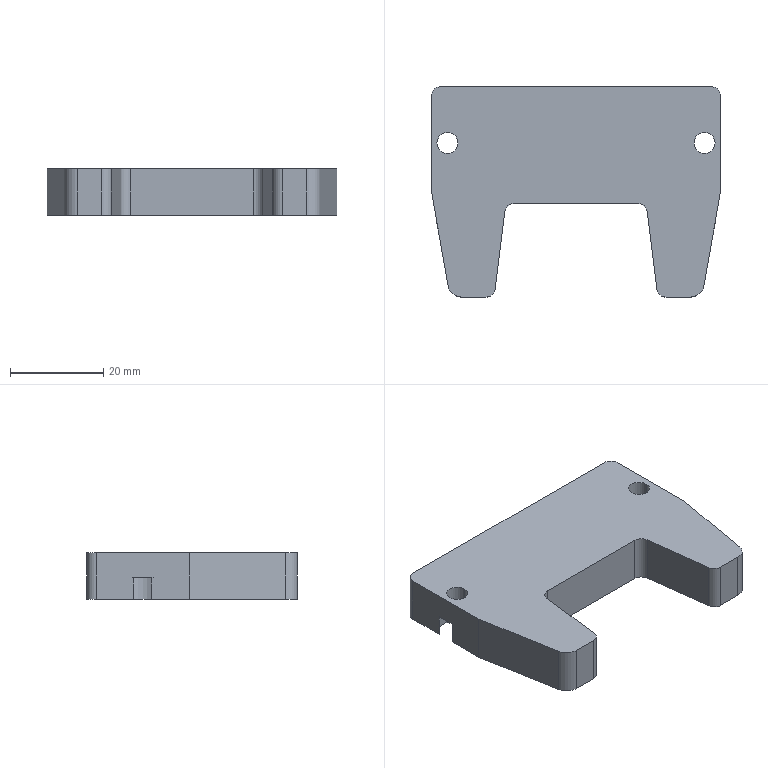Part | SolidWorks | features BaseBody 1 | 1 solid | 29 faces | box 62 x 45 x 10 mm | volume 19803 mm3 | cylinder 15 | plane 14 | commonest cylinder face diameters 4 x6 4.5 x4 8 x3 6 x2
STEP:
#1=CARTESIAN_POINT('',(-25.25,10.5,10.));
#2=VERTEX_POINT('',#1);
#3=CARTESIAN_POINT('',(-25.25,10.5,4.6));
#4=VERTEX_POINT('',#3);
#5=CARTESIAN_POINT('',(-25.25,10.5,0.));
#6=DIRECTION('',(0.,0.,-1.));
#7=VECTOR('',#6,1000.);
#8=LINE('',#5,#7);
#9=EDGE_CURVE('',#2,#4,#8,.T.);
#10=ORIENTED_EDGE('',*,*,#9,.F.);
#11=CARTESIAN_POINT('',(-29.75,10.5,10.));
#12=VERTEX_POINT('',#11);
#13=CARTESIAN_POINT('',(-27.5,10.5,10.));
#14=DIRECTION('',(0.,0.,1.));
#15=DIRECTION('',(1.,0.,0.));
#16=AXIS2_PLACEMENT_3D('',#13,#14,#15);
#17=CIRCLE('',#16,2.25);
#18=EDGE_CURVE('',#2,#12,#17,.T.);
#19=ORIENTED_EDGE('',*,*,#18,.T.);
#20=CARTESIAN_POINT('',(-29.75,10.5,4.6));
#21=VERTEX_POINT('',#20);
#22=CARTESIAN_POINT('',(-29.75,10.5,0.));
#23=DIRECTION('',(0.,0.,-1.));
#24=VECTOR('',#23,1000.);
#25=LINE('',#22,#24);
#26=EDGE_CURVE('',#12,#21,#25,.T.);
#27=ORIENTED_EDGE('',*,*,#26,.T.);
#28=CARTESIAN_POINT('',(-27.5,10.5,4.6));
#29=DIRECTION('',(0.,0.,-1.));
#30=DIRECTION('',(-1.,0.,0.));
#31=AXIS2_PLACEMENT_3D('',#28,#29,#30);
#32=CIRCLE('',#31,2.25);
#33=EDGE_CURVE('',#21,#4,#32,.T.);
#34=ORIENTED_EDGE('',*,*,#33,.T.);
#35=EDGE_LOOP('',(#10,#19,#27,#34));
#36=FACE_OUTER_BOUND('',#35,.T.);
#37=CARTESIAN_POINT('',(-27.5,10.5,0.));
#38=DIRECTION('',(0.,0.,-1.));
#39=DIRECTION('',(-1.,0.,0.));
#40=AXIS2_PLACEMENT_3D('',#37,#38,#39);
#41=CYLINDRICAL_SURFACE('',#40,2.25);
#42=ADVANCED_FACE('',(#36),#41,.F.);
#43=CARTESIAN_POINT('',(-31.,12.436,4.6));
#44=VERTEX_POINT('',#43);
#45=CARTESIAN_POINT('',(-31.,8.564,4.6));
#46=VERTEX_POINT('',#45);
#47=CARTESIAN_POINT('',(-27.5,10.5,4.6));
#48=DIRECTION('',(0.,0.,-1.));
#49=DIRECTION('',(-1.,0.,0.));
#50=AXIS2_PLACEMENT_3D('',#47,#48,#49);
#51=CIRCLE('',#50,4.);
#52=EDGE_CURVE('',#44,#46,#51,.T.);
#53=ORIENTED_EDGE('',*,*,#52,.F.);
#54=CARTESIAN_POINT('',(-31.,12.436,0.));
#55=VERTEX_POINT('',#54);
#56=CARTESIAN_POINT('',(-31.,12.436,0.));
#57=DIRECTION('',(0.,0.,1.));
#58=VECTOR('',#57,1000.);
#59=LINE('',#56,#58);
#60=EDGE_CURVE('',#55,#44,#59,.T.);
#61=ORIENTED_EDGE('',*,*,#60,.F.);
#62=CARTESIAN_POINT('',(-31.,8.564,0.));
#63=VERTEX_POINT('',#62);
#64=CARTESIAN_POINT('',(-27.5,10.5,0.));
#65=DIRECTION('',(0.,0.,-1.));
#66=DIRECTION('',(-1.,0.,0.));
#67=AXIS2_PLACEMENT_3D('',#64,#65,#66);
#68=CIRCLE('',#67,4.);
#69=EDGE_CURVE('',#55,#63,#68,.T.);
#70=ORIENTED_EDGE('',*,*,#69,.T.);
#71=CARTESIAN_POINT('',(-31.,8.564,0.));
#72=DIRECTION('',(0.,0.,-1.));
#73=VECTOR('',#72,1000.);
#74=LINE('',#71,#73);
#75=EDGE_CURVE('',#46,#63,#74,.T.);
#76=ORIENTED_EDGE('',*,*,#75,.F.);
#77=EDGE_LOOP('',(#53,#61,#70,#76));
#78=FACE_OUTER_BOUND('',#77,.T.);
#79=CARTESIAN_POINT('',(-27.5,10.5,0.));
#80=DIRECTION('',(0.,0.,-1.));
#81=DIRECTION('',(-1.,0.,0.));
#82=AXIS2_PLACEMENT_3D('',#79,#80,#81);
#83=CYLINDRICAL_SURFACE('',#82,4.);
#84=ADVANCED_FACE('',(#78),#83,.F.);
#85=ORIENTED_EDGE('',*,*,#33,.F.);
#86=CARTESIAN_POINT('',(-27.5,10.5,4.6));
#87=DIRECTION('',(0.,0.,-1.));
#88=DIRECTION('',(-1.,0.,0.));
#89=AXIS2_PLACEMENT_3D('',#86,#87,#88);
#90=CIRCLE('',#89,2.25);
#91=EDGE_CURVE('',#4,#21,#90,.T.);
#92=ORIENTED_EDGE('',*,*,#91,.F.);
#93=EDGE_LOOP('',(#85,#92));
#94=FACE_BOUND('',#93,.T.);
#95=ORIENTED_EDGE('',*,*,#52,.T.);
#96=CARTESIAN_POINT('',(-31.,-22.5,4.6));
#97=DIRECTION('',(0.,-1.,0.));
#98=VECTOR('',#97,1000.);
#99=LINE('',#96,#98);
#100=EDGE_CURVE('',#44,#46,#99,.T.);
#101=ORIENTED_EDGE('',*,*,#100,.F.);
#102=EDGE_LOOP('',(#95,#101));
#103=FACE_OUTER_BOUND('',#102,.T.);
#104=CARTESIAN_POINT('',(-25.25,10.5,4.6));
#105=DIRECTION('',(0.,0.,1.));
#106=DIRECTION('',(1.,0.,0.));
#107=AXIS2_PLACEMENT_3D('',#104,#105,#106);
#108=PLANE('',#107);
#109=ADVANCED_FACE('',(#94,#103),#108,.F.);
#110=CARTESIAN_POINT('',(29.75,10.5,10.));
#111=VERTEX_POINT('',#110);
#112=CARTESIAN_POINT('',(29.75,10.5,4.6));
#113=VERTEX_POINT('',#112);
#114=CARTESIAN_POINT('',(29.75,10.5,0.));
#115=DIRECTION('',(0.,0.,-1.));
#116=VECTOR('',#115,1000.);
#117=LINE('',#114,#116);
#118=EDGE_CURVE('',#111,#113,#117,.T.);
#119=ORIENTED_EDGE('',*,*,#118,.F.);
#120=CARTESIAN_POINT('',(25.25,10.5,10.));
#121=VERTEX_POINT('',#120);
#122=CARTESIAN_POINT('',(27.5,10.5,10.));
#123=DIRECTION('',(0.,0.,1.));
#124=DIRECTION('',(1.,0.,0.));
#125=AXIS2_PLACEMENT_3D('',#122,#123,#124);
#126=CIRCLE('',#125,2.25);
#127=EDGE_CURVE('',#111,#121,#126,.T.);
#128=ORIENTED_EDGE('',*,*,#127,.T.);
#129=CARTESIAN_POINT('',(25.25,10.5,4.6));
#130=VERTEX_POINT('',#129);
#131=CARTESIAN_POINT('',(25.25,10.5,0.));
#132=DIRECTION('',(0.,0.,-1.));
#133=VECTOR('',#132,1000.);
#134=LINE('',#131,#133);
#135=EDGE_CURVE('',#121,#130,#134,.T.);
#136=ORIENTED_EDGE('',*,*,#135,.T.);
#137=CARTESIAN_POINT('',(27.5,10.5,4.6));
#138=DIRECTION('',(0.,0.,-1.));
#139=DIRECTION('',(-1.,0.,0.));
#140=AXIS2_PLACEMENT_3D('',#137,#138,#139);
#141=CIRCLE('',#140,2.25);
#142=EDGE_CURVE('',#130,#113,#141,.T.);
#143=ORIENTED_EDGE('',*,*,#142,.T.);
#144=EDGE_LOOP('',(#119,#128,#136,#143));
#145=FACE_OUTER_BOUND('',#144,.T.);
#146=CARTESIAN_POINT('',(27.5,10.5,0.));
#147=DIRECTION('',(0.,0.,-1.));
#148=DIRECTION('',(-1.,0.,0.));
#149=AXIS2_PLACEMENT_3D('',#146,#147,#148);
#150=CYLINDRICAL_SURFACE('',#149,2.25);
#151=ADVANCED_FACE('',(#145),#150,.F.);
#152=CARTESIAN_POINT('',(23.5,10.5,4.6));
#153=VERTEX_POINT('',#152);
#154=CARTESIAN_POINT('',(23.5,10.5,0.));
#155=VERTEX_POINT('',#154);
#156=CARTESIAN_POINT('',(23.5,10.5,0.));
#157=DIRECTION('',(0.,0.,-1.));
#158=VECTOR('',#157,1000.);
#159=LINE('',#156,#158);
#160=EDGE_CURVE('',#153,#155,#159,.T.);
#161=ORIENTED_EDGE('',*,*,#160,.F.);
#162=CARTESIAN_POINT('',(31.,8.564,4.6));
#163=VERTEX_POINT('',#162);
#164=CARTESIAN_POINT('',(27.5,10.5,4.6));
#165=DIRECTION('',(0.,0.,-1.));
#166=DIRECTION('',(-1.,0.,0.));
#167=AXIS2_PLACEMENT_3D('',#164,#165,#166);
#168=CIRCLE('',#167,4.);
#169=EDGE_CURVE('',#163,#153,#168,.T.);
#170=ORIENTED_EDGE('',*,*,#169,.F.);
#171=CARTESIAN_POINT('',(31.,8.564,0.));
#172=VERTEX_POINT('',#171);
#173=CARTESIAN_POINT('',(31.,8.564,0.));
#174=DIRECTION('',(0.,0.,1.));
#175=VECTOR('',#174,1000.);
#176=LINE('',#173,#175);
#177=EDGE_CURVE('',#172,#163,#176,.T.);
#178=ORIENTED_EDGE('',*,*,#177,.F.);
#179=CARTESIAN_POINT('',(27.5,10.5,0.));
#180=DIRECTION('',(0.,0.,-1.));
#181=DIRECTION('',(-1.,0.,0.));
#182=AXIS2_PLACEMENT_3D('',#179,#180,#181);
#183=CIRCLE('',#182,4.);
#184=EDGE_CURVE('',#172,#155,#183,.T.);
#185=ORIENTED_EDGE('',*,*,#184,.T.);
#186=EDGE_LOOP('',(#161,#170,#178,#185));
#187=FACE_OUTER_BOUND('',#186,.T.);
#188=CARTESIAN_POINT('',(27.5,10.5,0.));
#189=DIRECTION('',(0.,0.,-1.));
#190=DIRECTION('',(-1.,0.,0.));
#191=AXIS2_PLACEMENT_3D('',#188,#189,#190);
#192=CYLINDRICAL_SURFACE('',#191,4.);
#193=ADVANCED_FACE('',(#187),#192,.F.);
#194=ORIENTED_EDGE('',*,*,#142,.F.);
#195=CARTESIAN_POINT('',(27.5,10.5,4.6));
#196=DIRECTION('',(0.,0.,-1.));
#197=DIRECTION('',(-1.,0.,0.));
#198=AXIS2_PLACEMENT_3D('',#195,#196,#197);
#199=CIRCLE('',#198,2.25);
#200=EDGE_CURVE('',#113,#130,#199,.T.);
#201=ORIENTED_EDGE('',*,*,#200,.F.);
#202=EDGE_LOOP('',(#194,#201));
#203=FACE_BOUND('',#202,.T.);
#204=ORIENTED_EDGE('',*,*,#169,.T.);
#205=CARTESIAN_POINT('',(31.,12.436,4.6));
#206=VERTEX_POINT('',#205);
#207=CARTESIAN_POINT('',(27.5,10.5,4.6));
#208=DIRECTION('',(0.,0.,-1.));
#209=DIRECTION('',(-1.,0.,0.));
#210=AXIS2_PLACEMENT_3D('',#207,#208,#209);
#211=CIRCLE('',#210,4.);
#212=EDGE_CURVE('',#153,#206,#211,.T.);
#213=ORIENTED_EDGE('',*,*,#212,.T.);
#214=CARTESIAN_POINT('',(31.,-22.5,4.6));
#215=DIRECTION('',(0.,1.,0.));
#216=VECTOR('',#215,1000.);
#217=LINE('',#214,#216);
#218=EDGE_CURVE('',#163,#206,#217,.T.);
#219=ORIENTED_EDGE('',*,*,#218,.F.);
#220=EDGE_LOOP('',(#204,#213,#219));
#221=FACE_OUTER_BOUND('',#220,.T.);
#222=CARTESIAN_POINT('',(29.75,10.5,4.6));
#223=DIRECTION('',(0.,0.,1.));
#224=DIRECTION('',(1.,0.,0.));
#225=AXIS2_PLACEMENT_3D('',#222,#223,#224);
#226=PLANE('',#225);
#227=ADVANCED_FACE('',(#203,#221),#226,.F.);
#228=CARTESIAN_POINT('',(-27.382,-20.021,10.));
#229=VERTEX_POINT('',#228);
#230=CARTESIAN_POINT('',(-24.427,-22.5,10.));
#231=VERTEX_POINT('',#230);
#232=CARTESIAN_POINT('',(-24.427,-19.5,10.));
#233=DIRECTION('',(0.,0.,1.));
#234=DIRECTION('',(1.,0.,0.));
#235=AXIS2_PLACEMENT_3D('',#232,#233,#234);
#236=CIRCLE('',#235,3.);
#237=EDGE_CURVE('',#229,#231,#236,.T.);
#238=ORIENTED_EDGE('',*,*,#237,.F.);
#239=CARTESIAN_POINT('',(-27.382,-20.021,0.));
#240=VERTEX_POINT('',#239);
#241=CARTESIAN_POINT('',(-27.382,-20.021,10.));
#242=DIRECTION('',(0.,0.,1.));
#243=VECTOR('',#242,1000.);
#244=LINE('',#241,#243);
#245=EDGE_CURVE('',#240,#229,#244,.T.);
#246=ORIENTED_EDGE('',*,*,#245,.F.);
#247=CARTESIAN_POINT('',(-24.427,-22.5,0.));
#248=VERTEX_POINT('',#247);
#249=CARTESIAN_POINT('',(-24.427,-19.5,0.));
#250=DIRECTION('',(0.,0.,-1.));
#251=DIRECTION('',(1.,0.,0.));
#252=AXIS2_PLACEMENT_3D('',#249,#250,#251);
#253=CIRCLE('',#252,3.);
#254=EDGE_CURVE('',#248,#240,#253,.T.);
#255=ORIENTED_EDGE('',*,*,#254,.F.);
#256=CARTESIAN_POINT('',(-24.427,-22.5,0.));
#257=DIRECTION('',(0.,0.,-1.));
#258=VECTOR('',#257,1000.);
#259=LINE('',#256,#258);
#260=EDGE_CURVE('',#231,#248,#259,.T.);
#261=ORIENTED_EDGE('',*,*,#260,.F.);
#262=EDGE_LOOP('',(#238,#246,#255,#261));
#263=FACE_OUTER_BOUND('',#262,.T.);
#264=CARTESIAN_POINT('',(-24.427,-19.5,10.));
#265=DIRECTION('',(0.,0.,-1.));
#266=DIRECTION('',(-1.,0.,0.));
#267=AXIS2_PLACEMENT_3D('',#264,#265,#266);
#268=CYLINDRICAL_SURFACE('',#267,3.);
#269=ADVANCED_FACE('',(#263),#268,.T.);
#270=CARTESIAN_POINT('',(27.382,-20.021,0.));
#271=VERTEX_POINT('',#270);
#272=CARTESIAN_POINT('',(24.427,-22.5,0.));
#273=VERTEX_POINT('',#272);
#274=CARTESIAN_POINT('',(24.427,-19.5,0.));
#275=DIRECTION('',(0.,0.,-1.));
#276=DIRECTION('',(1.,0.,0.));
#277=AXIS2_PLACEMENT_3D('',#274,#275,#276);
#278=CIRCLE('',#277,3.);
#279=EDGE_CURVE('',#271,#273,#278,.T.);
#280=ORIENTED_EDGE('',*,*,#279,.F.);
#281=CARTESIAN_POINT('',(27.382,-20.021,10.));
#282=VERTEX_POINT('',#281);
#283=CARTESIAN_POINT('',(27.382,-20.021,0.));
#284=DIRECTION('',(0.,0.,-1.));
#285=VECTOR('',#284,1000.);
#286=LINE('',#283,#285);
#287=EDGE_CURVE('',#282,#271,#286,.T.);
#288=ORIENTED_EDGE('',*,*,#287,.F.);
#289=CARTESIAN_POINT('',(24.427,-22.5,10.));
#290=VERTEX_POINT('',#289);
#291=CARTESIAN_POINT('',(24.427,-19.5,10.));
#292=DIRECTION('',(0.,0.,1.));
#293=DIRECTION('',(1.,0.,0.));
#294=AXIS2_PLACEMENT_3D('',#291,#292,#293);
#295=CIRCLE('',#294,3.);
#296=EDGE_CURVE('',#290,#282,#295,.T.);
#297=ORIENTED_EDGE('',*,*,#296,.F.);
#298=CARTESIAN_POINT('',(24.427,-22.5,10.));
#299=DIRECTION('',(0.,0.,1.));
#300=VECTOR('',#299,1000.);
#301=LINE('',#298,#300);
#302=EDGE_CURVE('',#273,#290,#301,.T.);
#303=ORIENTED_EDGE('',*,*,#302,.F.);
#304=EDGE_LOOP('',(#280,#288,#297,#303));
#305=FACE_OUTER_BOUND('',#304,.T.);
#306=CARTESIAN_POINT('',(24.427,-19.5,10.));
#307=DIRECTION('',(0.,0.,1.));
#308=DIRECTION('',(1.,0.,0.));
#309=AXIS2_PLACEMENT_3D('',#306,#307,#308);
#310=CYLINDRICAL_SURFACE('',#309,3.);
#311=ADVANCED_FACE('',(#305),#310,.T.);
#312=CARTESIAN_POINT('',(-31.,0.5,0.));
#313=VERTEX_POINT('',#312);
#314=CARTESIAN_POINT('',(-26.944,-22.5,0.));
#315=DIRECTION('',(-0.1736,0.9848,0.));
#316=VECTOR('',#315,1000.);
#317=LINE('',#314,#316);
#318=EDGE_CURVE('',#240,#313,#317,.T.);
#319=ORIENTED_EDGE('',*,*,#318,.F.);
#320=ORIENTED_EDGE('',*,*,#245,.T.);
#321=CARTESIAN_POINT('',(-31.,0.5,10.));
#322=VERTEX_POINT('',#321);
#323=CARTESIAN_POINT('',(-29.98,-5.286,10.));
#324=DIRECTION('',(0.1736,-0.9848,0.));
#325=VECTOR('',#324,1000.);
#326=LINE('',#323,#325);
#327=EDGE_CURVE('',#322,#229,#326,.T.);
#328=ORIENTED_EDGE('',*,*,#327,.F.);
#329=CARTESIAN_POINT('',(-31.,0.5,10.));
#330=DIRECTION('',(0.,0.,1.));
#331=VECTOR('',#330,1000.);
#332=LINE('',#329,#331);
#333=EDGE_CURVE('',#313,#322,#332,.T.);
#334=ORIENTED_EDGE('',*,*,#333,.F.);
#335=EDGE_LOOP('',(#319,#320,#328,#334));
#336=FACE_OUTER_BOUND('',#335,.T.);
#337=CARTESIAN_POINT('',(-26.944,-22.5,10.));
#338=DIRECTION('',(0.9848,0.1736,0.));
#339=DIRECTION('',(0.,0.,-1.));
#340=AXIS2_PLACEMENT_3D('',#337,#338,#339);
#341=PLANE('',#340);
#342=ADVANCED_FACE('',(#336),#341,.F.);
#343=CARTESIAN_POINT('',(31.,0.5,10.));
#344=VERTEX_POINT('',#343);
#345=CARTESIAN_POINT('',(29.98,-5.286,10.));
#346=DIRECTION('',(0.1736,0.9848,0.));
#347=VECTOR('',#346,1000.);
#348=LINE('',#345,#347);
#349=EDGE_CURVE('',#282,#344,#348,.T.);
#350=ORIENTED_EDGE('',*,*,#349,.F.);
#351=ORIENTED_EDGE('',*,*,#287,.T.);
#352=CARTESIAN_POINT('',(31.,0.5,0.));
#353=VERTEX_POINT('',#352);
#354=CARTESIAN_POINT('',(31.,0.5,0.));
#355=DIRECTION('',(-0.1736,-0.9848,0.));
#356=VECTOR('',#355,1000.);
#357=LINE('',#354,#356);
#358=EDGE_CURVE('',#353,#271,#357,.T.);
#359=ORIENTED_EDGE('',*,*,#358,.F.);
#360=CARTESIAN_POINT('',(31.,0.5,10.));
#361=DIRECTION('',(0.,0.,-1.));
#362=VECTOR('',#361,1000.);
#363=LINE('',#360,#362);
#364=EDGE_CURVE('',#344,#353,#363,.T.);
#365=ORIENTED_EDGE('',*,*,#364,.F.);
#366=EDGE_LOOP('',(#350,#351,#359,#365));
#367=FACE_OUTER_BOUND('',#366,.T.);
#368=CARTESIAN_POINT('',(31.,0.5,10.));
#369=DIRECTION('',(-0.9848,0.1736,0.));
#370=DIRECTION('',(0.,0.,1.));
#371=AXIS2_PLACEMENT_3D('',#368,#369,#370);
#372=PLANE('',#371);
#373=ADVANCED_FACE('',(#367),#372,.F.);
#374=CARTESIAN_POINT('',(-13.234,-2.5,0.));
#375=VERTEX_POINT('',#374);
#376=CARTESIAN_POINT('',(-15.219,-4.252,0.));
#377=VERTEX_POINT('',#376);
#378=CARTESIAN_POINT('',(-13.234,-4.5,0.));
#379=DIRECTION('',(0.,0.,1.));
#380=DIRECTION('',(1.,0.,0.));
#381=AXIS2_PLACEMENT_3D('',#378,#379,#380);
#382=CIRCLE('',#381,2.);
#383=EDGE_CURVE('',#375,#377,#382,.T.);
#384=ORIENTED_EDGE('',*,*,#383,.F.);
#385=CARTESIAN_POINT('',(-13.234,-2.5,10.));
#386=VERTEX_POINT('',#385);
#387=CARTESIAN_POINT('',(-13.234,-2.5,0.));
#388=DIRECTION('',(0.,0.,-1.));
#389=VECTOR('',#388,1000.);
#390=LINE('',#387,#389);
#391=EDGE_CURVE('',#386,#375,#390,.T.);
#392=ORIENTED_EDGE('',*,*,#391,.F.);
#393=CARTESIAN_POINT('',(-15.219,-4.252,10.));
#394=VERTEX_POINT('',#393);
#395=CARTESIAN_POINT('',(-13.234,-4.5,10.));
#396=DIRECTION('',(0.,0.,-1.));
#397=DIRECTION('',(1.,0.,0.));
#398=AXIS2_PLACEMENT_3D('',#395,#396,#397);
#399=CIRCLE('',#398,2.);
#400=EDGE_CURVE('',#394,#386,#399,.T.);
#401=ORIENTED_EDGE('',*,*,#400,.F.);
#402=CARTESIAN_POINT('',(-15.219,-4.252,10.));
#403=DIRECTION('',(0.,0.,1.));
#404=VECTOR('',#403,1000.);
#405=LINE('',#402,#404);
#406=EDGE_CURVE('',#377,#394,#405,.T.);
#407=ORIENTED_EDGE('',*,*,#406,.F.);
#408=EDGE_LOOP('',(#384,#392,#401,#407));
#409=FACE_OUTER_BOUND('',#408,.T.);
#410=CARTESIAN_POINT('',(-13.234,-4.5,-0.001));
#411=DIRECTION('',(0.,0.,-1.));
#412=DIRECTION('',(-1.,0.,0.));
#413=AXIS2_PLACEMENT_3D('',#410,#411,#412);
#414=CYLINDRICAL_SURFACE('',#413,2.);
#415=ADVANCED_FACE('',(#409),#414,.F.);
#416=CARTESIAN_POINT('',(15.219,-4.252,0.));
#417=VERTEX_POINT('',#416);
#418=CARTESIAN_POINT('',(13.234,-2.5,0.));
#419=VERTEX_POINT('',#418);
#420=CARTESIAN_POINT('',(13.234,-4.5,0.));
#421=DIRECTION('',(0.,0.,1.));
#422=DIRECTION('',(1.,0.,0.));
#423=AXIS2_PLACEMENT_3D('',#420,#421,#422);
#424=CIRCLE('',#423,2.);
#425=EDGE_CURVE('',#417,#419,#424,.T.);
#426=ORIENTED_EDGE('',*,*,#425,.F.);
#427=CARTESIAN_POINT('',(15.219,-4.252,10.));
#428=VERTEX_POINT('',#427);
#429=CARTESIAN_POINT('',(15.219,-4.252,0.));
#430=DIRECTION('',(0.,0.,-1.));
#431=VECTOR('',#430,1000.);
#432=LINE('',#429,#431);
#433=EDGE_CURVE('',#428,#417,#432,.T.);
#434=ORIENTED_EDGE('',*,*,#433,.F.);
#435=CARTESIAN_POINT('',(13.234,-2.5,10.));
#436=VERTEX_POINT('',#435);
#437=CARTESIAN_POINT('',(13.234,-4.5,10.));
#438=DIRECTION('',(0.,0.,-1.));
#439=DIRECTION('',(1.,0.,0.));
#440=AXIS2_PLACEMENT_3D('',#437,#438,#439);
#441=CIRCLE('',#440,2.);
#442=EDGE_CURVE('',#436,#428,#441,.T.);
#443=ORIENTED_EDGE('',*,*,#442,.F.);
#444=CARTESIAN_POINT('',(13.234,-2.5,10.));
#445=DIRECTION('',(0.,0.,1.));
#446=VECTOR('',#445,1000.);
#447=LINE('',#444,#446);
#448=EDGE_CURVE('',#419,#436,#447,.T.);
#449=ORIENTED_EDGE('',*,*,#448,.F.);
#450=EDGE_LOOP('',(#426,#434,#443,#449));
#451=FACE_OUTER_BOUND('',#450,.T.);
#452=CARTESIAN_POINT('',(13.234,-4.5,-0.001));
#453=DIRECTION('',(0.,0.,-1.));
#454=DIRECTION('',(-1.,0.,0.));
#455=AXIS2_PLACEMENT_3D('',#452,#453,#454);
#456=CYLINDRICAL_SURFACE('',#455,2.);
#457=ADVANCED_FACE('',(#451),#456,.F.);
#458=CARTESIAN_POINT('',(-17.281,-20.748,0.));
#459=VERTEX_POINT('',#458);
#460=CARTESIAN_POINT('',(-19.266,-22.5,0.));
#461=VERTEX_POINT('',#460);
#462=CARTESIAN_POINT('',(-19.266,-20.5,0.));
#463=DIRECTION('',(0.,0.,-1.));
#464=DIRECTION('',(1.,0.,0.));
#465=AXIS2_PLACEMENT_3D('',#462,#463,#464);
#466=CIRCLE('',#465,2.);
#467=EDGE_CURVE('',#459,#461,#466,.T.);
#468=ORIENTED_EDGE('',*,*,#467,.F.);
#469=CARTESIAN_POINT('',(-17.281,-20.748,10.));
#470=VERTEX_POINT('',#469);
#471=CARTESIAN_POINT('',(-17.281,-20.748,-0.001));
#472=DIRECTION('',(0.,0.,-1.));
#473=VECTOR('',#472,1000.);
#474=LINE('',#471,#473);
#475=EDGE_CURVE('',#470,#459,#474,.T.);
#476=ORIENTED_EDGE('',*,*,#475,.F.);
#477=CARTESIAN_POINT('',(-19.266,-22.5,10.));
#478=VERTEX_POINT('',#477);
#479=CARTESIAN_POINT('',(-19.266,-20.5,10.));
#480=DIRECTION('',(0.,0.,1.));
#481=DIRECTION('',(1.,0.,0.));
#482=AXIS2_PLACEMENT_3D('',#479,#480,#481);
#483=CIRCLE('',#482,2.);
#484=EDGE_CURVE('',#478,#470,#483,.T.);
#485=ORIENTED_EDGE('',*,*,#484,.F.);
#486=CARTESIAN_POINT('',(-19.266,-22.5,10.));
#487=DIRECTION('',(0.,0.,1.));
#488=VECTOR('',#487,1000.);
#489=LINE('',#486,#488);
#490=EDGE_CURVE('',#461,#478,#489,.T.);
#491=ORIENTED_EDGE('',*,*,#490,.F.);
#492=EDGE_LOOP('',(#468,#476,#485,#491));
#493=FACE_OUTER_BOUND('',#492,.T.);
#494=CARTESIAN_POINT('',(-19.266,-20.5,10.));
#495=DIRECTION('',(0.,0.,1.));
#496=DIRECTION('',(1.,0.,0.));
#497=AXIS2_PLACEMENT_3D('',#494,#495,#496);
#498=CYLINDRICAL_SURFACE('',#497,2.);
#499=ADVANCED_FACE('',(#493),#498,.T.);
#500=CARTESIAN_POINT('',(19.266,-22.5,0.));
#501=VERTEX_POINT('',#500);
#502=CARTESIAN_POINT('',(17.281,-20.748,0.));
#503=VERTEX_POINT('',#502);
#504=CARTESIAN_POINT('',(19.266,-20.5,0.));
#505=DIRECTION('',(0.,0.,-1.));
#506=DIRECTION('',(1.,0.,0.));
#507=AXIS2_PLACEMENT_3D('',#504,#505,#506);
#508=CIRCLE('',#507,2.);
#509=EDGE_CURVE('',#501,#503,#508,.T.);
#510=ORIENTED_EDGE('',*,*,#509,.F.);
#511=CARTESIAN_POINT('',(19.266,-22.5,10.));
#512=VERTEX_POINT('',#511);
#513=CARTESIAN_POINT('',(19.266,-22.5,10.));
#514=DIRECTION('',(0.,0.,-1.));
#515=VECTOR('',#514,1000.);
#516=LINE('',#513,#515);
#517=EDGE_CURVE('',#512,#501,#516,.T.);
#518=ORIENTED_EDGE('',*,*,#517,.F.);
#519=CARTESIAN_POINT('',(17.281,-20.748,10.));
#520=VERTEX_POINT('',#519);
#521=CARTESIAN_POINT('',(19.266,-20.5,10.));
#522=DIRECTION('',(0.,0.,1.));
#523=DIRECTION('',(1.,0.,0.));
#524=AXIS2_PLACEMENT_3D('',#521,#522,#523);
#525=CIRCLE('',#524,2.);
#526=EDGE_CURVE('',#520,#512,#525,.T.);
#527=ORIENTED_EDGE('',*,*,#526,.F.);
#528=CARTESIAN_POINT('',(17.281,-20.748,-0.001));
#529=DIRECTION('',(0.,0.,1.));
#530=VECTOR('',#529,1000.);
#531=LINE('',#528,#530);
#532=EDGE_CURVE('',#503,#520,#531,.T.);
#533=ORIENTED_EDGE('',*,*,#532,.F.);
#534=EDGE_LOOP('',(#510,#518,#527,#533));
#535=FACE_OUTER_BOUND('',#534,.T.);
#536=CARTESIAN_POINT('',(19.266,-20.5,-0.001));
#537=DIRECTION('',(0.,0.,1.));
#538=DIRECTION('',(1.,0.,0.));
#539=AXIS2_PLACEMENT_3D('',#536,#537,#538);
#540=CYLINDRICAL_SURFACE('',#539,2.);
#541=ADVANCED_FACE('',(#535),#540,.T.);
#542=CARTESIAN_POINT('',(31.,20.5,10.));
#543=VERTEX_POINT('',#542);
#544=CARTESIAN_POINT('',(29.,22.5,10.));
#545=VERTEX_POINT('',#544);
#546=CARTESIAN_POINT('',(29.,20.5,10.));
#547=DIRECTION('',(0.,0.,1.));
#548=DIRECTION('',(1.,0.,0.));
#549=AXIS2_PLACEMENT_3D('',#546,#547,#548);
#550=CIRCLE('',#549,2.);
#551=EDGE_CURVE('',#543,#545,#550,.T.);
#552=ORIENTED_EDGE('',*,*,#551,.F.);
#553=CARTESIAN_POINT('',(31.,20.5,0.));
#554=VERTEX_POINT('',#553);
#555=CARTESIAN_POINT('',(31.,20.5,10.));
#556=DIRECTION('',(0.,0.,1.));
#557=VECTOR('',#556,1000.);
#558=LINE('',#555,#557);
#559=EDGE_CURVE('',#554,#543,#558,.T.);
#560=ORIENTED_EDGE('',*,*,#559,.F.);
#561=CARTESIAN_POINT('',(29.,22.5,0.));
#562=VERTEX_POINT('',#561);
#563=CARTESIAN_POINT('',(29.,20.5,0.));
#564=DIRECTION('',(0.,0.,-1.));
#565=DIRECTION('',(1.,0.,0.));
#566=AXIS2_PLACEMENT_3D('',#563,#564,#565);
#567=CIRCLE('',#566,2.);
#568=EDGE_CURVE('',#562,#554,#567,.T.);
#569=ORIENTED_EDGE('',*,*,#568,.F.);
#570=CARTESIAN_POINT('',(29.,22.5,10.));
#571=DIRECTION('',(0.,0.,-1.));
#572=VECTOR('',#571,1000.);
#573=LINE('',#570,#572);
#574=EDGE_CURVE('',#545,#562,#573,.T.);
#575=ORIENTED_EDGE('',*,*,#574,.F.);
#576=EDGE_LOOP('',(#552,#560,#569,#575));
#577=FACE_OUTER_BOUND('',#576,.T.);
#578=CARTESIAN_POINT('',(29.,20.5,10.));
#579=DIRECTION('',(0.,0.,-1.));
#580=DIRECTION('',(-1.,0.,0.));
#581=AXIS2_PLACEMENT_3D('',#578,#579,#580);
#582=CYLINDRICAL_SURFACE('',#581,2.);
#583=ADVANCED_FACE('',(#577),#582,.T.);
#584=CARTESIAN_POINT('',(-29.,22.5,10.));
#585=VERTEX_POINT('',#584);
#586=CARTESIAN_POINT('',(-31.,20.5,10.));
#587=VERTEX_POINT('',#586);
#588=CARTESIAN_POINT('',(-29.,20.5,10.));
#589=DIRECTION('',(0.,0.,1.));
#590=DIRECTION('',(1.,0.,0.));
#591=AXIS2_PLACEMENT_3D('',#588,#589,#590);
#592=CIRCLE('',#591,2.);
#593=EDGE_CURVE('',#585,#587,#592,.T.);
#594=ORIENTED_EDGE('',*,*,#593,.F.);
#595=CARTESIAN_POINT('',(-29.,22.5,0.));
#596=VERTEX_POINT('',#595);
#597=CARTESIAN_POINT('',(-29.,22.5,10.));
#598=DIRECTION('',(0.,0.,1.));
#599=VECTOR('',#598,1000.);
#600=LINE('',#597,#599);
#601=EDGE_CURVE('',#596,#585,#600,.T.);
#602=ORIENTED_EDGE('',*,*,#601,.F.);
#603=CARTESIAN_POINT('',(-31.,20.5,0.));
#604=VERTEX_POINT('',#603);
#605=CARTESIAN_POINT('',(-29.,20.5,0.));
#606=DIRECTION('',(0.,0.,-1.));
#607=DIRECTION('',(1.,0.,0.));
#608=AXIS2_PLACEMENT_3D('',#605,#606,#607);
#609=CIRCLE('',#608,2.);
#610=EDGE_CURVE('',#604,#596,#609,.T.);
#611=ORIENTED_EDGE('',*,*,#610,.F.);
#612=CARTESIAN_POINT('',(-31.,20.5,10.));
#613=DIRECTION('',(0.,0.,-1.));
#614=VECTOR('',#613,1000.);
#615=LINE('',#612,#614);
#616=EDGE_CURVE('',#587,#604,#615,.T.);
#617=ORIENTED_EDGE('',*,*,#616,.F.);
#618=EDGE_LOOP('',(#594,#602,#611,#617));
#619=FACE_OUTER_BOUND('',#618,.T.);
#620=CARTESIAN_POINT('',(-29.,20.5,10.));
#621=DIRECTION('',(0.,0.,-1.));
#622=DIRECTION('',(-1.,0.,0.));
#623=AXIS2_PLACEMENT_3D('',#620,#621,#622);
#624=CYLINDRICAL_SURFACE('',#623,2.);
#625=ADVANCED_FACE('',(#619),#624,.T.);
#626=CARTESIAN_POINT('',(17.5,-22.5,0.));
#627=DIRECTION('',(0.124,-0.9923,0.));
#628=VECTOR('',#627,1000.);
#629=LINE('',#626,#628);
#630=EDGE_CURVE('',#417,#503,#629,.T.);
#631=ORIENTED_EDGE('',*,*,#630,.T.);
#632=ORIENTED_EDGE('',*,*,#532,.T.);
#633=CARTESIAN_POINT('',(17.5,-22.5,10.));
#634=DIRECTION('',(-0.124,0.9923,0.));
#635=VECTOR('',#634,1000.);
#636=LINE('',#633,#635);
#637=EDGE_CURVE('',#520,#428,#636,.T.);
#638=ORIENTED_EDGE('',*,*,#637,.T.);
#639=ORIENTED_EDGE('',*,*,#433,.T.);
#640=EDGE_LOOP('',(#631,#632,#638,#639));
#641=FACE_OUTER_BOUND('',#640,.T.);
#642=CARTESIAN_POINT('',(17.5,-22.5,-0.001));
#643=DIRECTION('',(0.9923,0.124,0.));
#644=DIRECTION('',(0.,0.,-1.));
#645=AXIS2_PLACEMENT_3D('',#642,#643,#644);
#646=PLANE('',#645);
#647=ADVANCED_FACE('',(#641),#646,.F.);
#648=CARTESIAN_POINT('',(15.,-2.5,0.));
#649=DIRECTION('',(1.,0.,0.));
#650=VECTOR('',#649,1000.);
#651=LINE('',#648,#650);
#652=EDGE_CURVE('',#375,#419,#651,.T.);
#653=ORIENTED_EDGE('',*,*,#652,.T.);
#654=ORIENTED_EDGE('',*,*,#448,.T.);
#655=CARTESIAN_POINT('',(15.,-2.5,10.));
#656=DIRECTION('',(-1.,0.,0.));
#657=VECTOR('',#656,1000.);
#658=LINE('',#655,#657);
#659=EDGE_CURVE('',#436,#386,#658,.T.);
#660=ORIENTED_EDGE('',*,*,#659,.T.);
#661=ORIENTED_EDGE('',*,*,#391,.T.);
#662=EDGE_LOOP('',(#653,#654,#660,#661));
#663=FACE_OUTER_BOUND('',#662,.T.);
#664=CARTESIAN_POINT('',(15.,-2.5,-0.001));
#665=DIRECTION('',(0.,1.,0.));
#666=DIRECTION('',(1.,0.,0.));
#667=AXIS2_PLACEMENT_3D('',#664,#665,#666);
#668=PLANE('',#667);
#669=ADVANCED_FACE('',(#663),#668,.F.);
#670=CARTESIAN_POINT('',(-15.,-2.5,10.));
#671=DIRECTION('',(-0.124,-0.9923,0.));
#672=VECTOR('',#671,1000.);
#673=LINE('',#670,#672);
#674=EDGE_CURVE('',#394,#470,#673,.T.);
#675=ORIENTED_EDGE('',*,*,#674,.T.);
#676=ORIENTED_EDGE('',*,*,#475,.T.);
#677=CARTESIAN_POINT('',(-15.,-2.5,0.));
#678=DIRECTION('',(0.124,0.9923,0.));
#679=VECTOR('',#678,1000.);
#680=LINE('',#677,#679);
#681=EDGE_CURVE('',#459,#377,#680,.T.);
#682=ORIENTED_EDGE('',*,*,#681,.T.);
#683=ORIENTED_EDGE('',*,*,#406,.T.);
#684=EDGE_LOOP('',(#675,#676,#682,#683));
#685=FACE_OUTER_BOUND('',#684,.T.);
#686=CARTESIAN_POINT('',(-15.,-2.5,-0.001));
#687=DIRECTION('',(-0.9923,0.124,0.));
#688=DIRECTION('',(0.,0.,1.));
#689=AXIS2_PLACEMENT_3D('',#686,#687,#688);
#690=PLANE('',#689);
#691=ADVANCED_FACE('',(#685),#690,.F.);
#692=CARTESIAN_POINT('',(27.5,10.5,10.));
#693=DIRECTION('',(0.,0.,1.));
#694=DIRECTION('',(1.,0.,0.));
#695=AXIS2_PLACEMENT_3D('',#692,#693,#694);
#696=CIRCLE('',#695,2.25);
#697=EDGE_CURVE('',#121,#111,#696,.T.);
#698=ORIENTED_EDGE('',*,*,#697,.F.);
#699=ORIENTED_EDGE('',*,*,#127,.F.);
#700=EDGE_LOOP('',(#698,#699));
#701=FACE_BOUND('',#700,.T.);
#702=CARTESIAN_POINT('',(-27.5,10.5,10.));
#703=DIRECTION('',(0.,0.,1.));
#704=DIRECTION('',(1.,0.,0.));
#705=AXIS2_PLACEMENT_3D('',#702,#703,#704);
#706=CIRCLE('',#705,2.25);
#707=EDGE_CURVE('',#12,#2,#706,.T.);
#708=ORIENTED_EDGE('',*,*,#707,.F.);
#709=ORIENTED_EDGE('',*,*,#18,.F.);
#710=EDGE_LOOP('',(#708,#709));
#711=FACE_BOUND('',#710,.T.);
#712=CARTESIAN_POINT('',(31.,-22.5,10.));
#713=DIRECTION('',(1.,0.,0.));
#714=VECTOR('',#713,1000.);
#715=LINE('',#712,#714);
#716=EDGE_CURVE('',#512,#290,#715,.T.);
#717=ORIENTED_EDGE('',*,*,#716,.T.);
#718=ORIENTED_EDGE('',*,*,#296,.T.);
#719=ORIENTED_EDGE('',*,*,#349,.T.);
#720=CARTESIAN_POINT('',(31.,-22.5,10.));
#721=DIRECTION('',(0.,1.,0.));
#722=VECTOR('',#721,1000.);
#723=LINE('',#720,#722);
#724=EDGE_CURVE('',#344,#543,#723,.T.);
#725=ORIENTED_EDGE('',*,*,#724,.T.);
#726=ORIENTED_EDGE('',*,*,#551,.T.);
#727=CARTESIAN_POINT('',(31.,22.5,10.));
#728=DIRECTION('',(-1.,0.,0.));
#729=VECTOR('',#728,1000.);
#730=LINE('',#727,#729);
#731=EDGE_CURVE('',#545,#585,#730,.T.);
#732=ORIENTED_EDGE('',*,*,#731,.T.);
#733=ORIENTED_EDGE('',*,*,#593,.T.);
#734=CARTESIAN_POINT('',(-31.,-22.5,10.));
#735=DIRECTION('',(0.,-1.,0.));
#736=VECTOR('',#735,1000.);
#737=LINE('',#734,#736);
#738=EDGE_CURVE('',#587,#322,#737,.T.);
#739=ORIENTED_EDGE('',*,*,#738,.T.);
#740=ORIENTED_EDGE('',*,*,#327,.T.);
#741=ORIENTED_EDGE('',*,*,#237,.T.);
#742=CARTESIAN_POINT('',(31.,-22.5,10.));
#743=DIRECTION('',(1.,0.,0.));
#744=VECTOR('',#743,1000.);
#745=LINE('',#742,#744);
#746=EDGE_CURVE('',#231,#478,#745,.T.);
#747=ORIENTED_EDGE('',*,*,#746,.T.);
#748=ORIENTED_EDGE('',*,*,#484,.T.);
#749=ORIENTED_EDGE('',*,*,#674,.F.);
#750=ORIENTED_EDGE('',*,*,#400,.T.);
#751=ORIENTED_EDGE('',*,*,#659,.F.);
#752=ORIENTED_EDGE('',*,*,#442,.T.);
#753=ORIENTED_EDGE('',*,*,#637,.F.);
#754=ORIENTED_EDGE('',*,*,#526,.T.);
#755=EDGE_LOOP('',(#717,#718,#719,#725,#726,#732,#733,#739,#740,#741,#747,#748,#749,#750,#751,#752,#753,#754));
#756=FACE_OUTER_BOUND('',#755,.T.);
#757=CARTESIAN_POINT('',(0.,0.,10.));
#758=DIRECTION('',(0.,0.,1.));
#759=DIRECTION('',(1.,0.,0.));
#760=AXIS2_PLACEMENT_3D('',#757,#758,#759);
#761=PLANE('',#760);
#762=ADVANCED_FACE('',(#701,#711,#756),#761,.T.);
#763=CARTESIAN_POINT('',(31.,22.5,0.));
#764=DIRECTION('',(-1.,0.,0.));
#765=VECTOR('',#764,1000.);
#766=LINE('',#763,#765);
#767=EDGE_CURVE('',#562,#596,#766,.T.);
#768=ORIENTED_EDGE('',*,*,#767,.T.);
#769=ORIENTED_EDGE('',*,*,#601,.T.);
#770=ORIENTED_EDGE('',*,*,#731,.F.);
#771=ORIENTED_EDGE('',*,*,#574,.T.);
#772=EDGE_LOOP('',(#768,#769,#770,#771));
#773=FACE_OUTER_BOUND('',#772,.T.);
#774=CARTESIAN_POINT('',(31.,22.5,10.));
#775=DIRECTION('',(0.,-1.,0.));
#776=DIRECTION('',(0.,0.,-1.));
#777=AXIS2_PLACEMENT_3D('',#774,#775,#776);
#778=PLANE('',#777);
#779=ADVANCED_FACE('',(#773),#778,.F.);
#780=ORIENTED_EDGE('',*,*,#218,.T.);
#781=CARTESIAN_POINT('',(31.,12.436,0.));
#782=VERTEX_POINT('',#781);
#783=CARTESIAN_POINT('',(31.,12.436,0.));
#784=DIRECTION('',(0.,0.,-1.));
#785=VECTOR('',#784,1000.);
#786=LINE('',#783,#785);
#787=EDGE_CURVE('',#206,#782,#786,.T.);
#788=ORIENTED_EDGE('',*,*,#787,.T.);
#789=CARTESIAN_POINT('',(31.,-22.5,0.));
#790=DIRECTION('',(0.,1.,0.));
#791=VECTOR('',#790,1000.);
#792=LINE('',#789,#791);
#793=EDGE_CURVE('',#782,#554,#792,.T.);
#794=ORIENTED_EDGE('',*,*,#793,.T.);
#795=ORIENTED_EDGE('',*,*,#559,.T.);
#796=ORIENTED_EDGE('',*,*,#724,.F.);
#797=ORIENTED_EDGE('',*,*,#364,.T.);
#798=CARTESIAN_POINT('',(31.,-22.5,0.));
#799=DIRECTION('',(0.,1.,0.));
#800=VECTOR('',#799,1000.);
#801=LINE('',#798,#800);
#802=EDGE_CURVE('',#353,#172,#801,.T.);
#803=ORIENTED_EDGE('',*,*,#802,.T.);
#804=ORIENTED_EDGE('',*,*,#177,.T.);
#805=EDGE_LOOP('',(#780,#788,#794,#795,#796,#797,#803,#804));
#806=FACE_OUTER_BOUND('',#805,.T.);
#807=CARTESIAN_POINT('',(31.,-22.5,10.));
#808=DIRECTION('',(-1.,0.,0.));
#809=DIRECTION('',(0.,0.,1.));
#810=AXIS2_PLACEMENT_3D('',#807,#808,#809);
#811=PLANE('',#810);
#812=ADVANCED_FACE('',(#806),#811,.F.);
#813=CARTESIAN_POINT('',(31.,-22.5,0.));
#814=DIRECTION('',(1.,0.,0.));
#815=VECTOR('',#814,1000.);
#816=LINE('',#813,#815);
#817=EDGE_CURVE('',#501,#273,#816,.T.);
#818=ORIENTED_EDGE('',*,*,#817,.T.);
#819=ORIENTED_EDGE('',*,*,#302,.T.);
#820=ORIENTED_EDGE('',*,*,#716,.F.);
#821=ORIENTED_EDGE('',*,*,#517,.T.);
#822=EDGE_LOOP('',(#818,#819,#820,#821));
#823=FACE_OUTER_BOUND('',#822,.T.);
#824=CARTESIAN_POINT('',(31.,-22.5,10.));
#825=DIRECTION('',(0.,1.,0.));
#826=DIRECTION('',(1.,0.,0.));
#827=AXIS2_PLACEMENT_3D('',#824,#825,#826);
#828=PLANE('',#827);
#829=ADVANCED_FACE('',(#823),#828,.F.);
#830=ORIENTED_EDGE('',*,*,#100,.T.);
#831=ORIENTED_EDGE('',*,*,#75,.T.);
#832=CARTESIAN_POINT('',(-31.,-22.5,0.));
#833=DIRECTION('',(0.,-1.,0.));
#834=VECTOR('',#833,1000.);
#835=LINE('',#832,#834);
#836=EDGE_CURVE('',#63,#313,#835,.T.);
#837=ORIENTED_EDGE('',*,*,#836,.T.);
#838=ORIENTED_EDGE('',*,*,#333,.T.);
#839=ORIENTED_EDGE('',*,*,#738,.F.);
#840=ORIENTED_EDGE('',*,*,#616,.T.);
#841=CARTESIAN_POINT('',(-31.,-22.5,0.));
#842=DIRECTION('',(0.,-1.,0.));
#843=VECTOR('',#842,1000.);
#844=LINE('',#841,#843);
#845=EDGE_CURVE('',#604,#55,#844,.T.);
#846=ORIENTED_EDGE('',*,*,#845,.T.);
#847=ORIENTED_EDGE('',*,*,#60,.T.);
#848=EDGE_LOOP('',(#830,#831,#837,#838,#839,#840,#846,#847));
#849=FACE_OUTER_BOUND('',#848,.T.);
#850=CARTESIAN_POINT('',(-31.,-22.5,10.));
#851=DIRECTION('',(1.,0.,0.));
#852=DIRECTION('',(0.,1.,0.));
#853=AXIS2_PLACEMENT_3D('',#850,#851,#852);
#854=PLANE('',#853);
#855=ADVANCED_FACE('',(#849),#854,.F.);
#856=ORIENTED_EDGE('',*,*,#746,.F.);
#857=ORIENTED_EDGE('',*,*,#260,.T.);
#858=CARTESIAN_POINT('',(31.,-22.5,0.));
#859=DIRECTION('',(1.,0.,0.));
#860=VECTOR('',#859,1000.);
#861=LINE('',#858,#860);
#862=EDGE_CURVE('',#248,#461,#861,.T.);
#863=ORIENTED_EDGE('',*,*,#862,.T.);
#864=ORIENTED_EDGE('',*,*,#490,.T.);
#865=EDGE_LOOP('',(#856,#857,#863,#864));
#866=FACE_OUTER_BOUND('',#865,.T.);
#867=CARTESIAN_POINT('',(31.,-22.5,10.));
#868=DIRECTION('',(0.,1.,0.));
#869=DIRECTION('',(1.,0.,0.));
#870=AXIS2_PLACEMENT_3D('',#867,#868,#869);
#871=PLANE('',#870);
#872=ADVANCED_FACE('',(#866),#871,.F.);
#873=ORIENTED_EDGE('',*,*,#69,.F.);
#874=ORIENTED_EDGE('',*,*,#845,.F.);
#875=ORIENTED_EDGE('',*,*,#610,.T.);
#876=ORIENTED_EDGE('',*,*,#767,.F.);
#877=ORIENTED_EDGE('',*,*,#568,.T.);
#878=ORIENTED_EDGE('',*,*,#793,.F.);
#879=CARTESIAN_POINT('',(27.5,10.5,0.));
#880=DIRECTION('',(0.,0.,-1.));
#881=DIRECTION('',(-1.,0.,0.));
#882=AXIS2_PLACEMENT_3D('',#879,#880,#881);
#883=CIRCLE('',#882,4.);
#884=EDGE_CURVE('',#155,#782,#883,.T.);
#885=ORIENTED_EDGE('',*,*,#884,.F.);
#886=ORIENTED_EDGE('',*,*,#184,.F.);
#887=ORIENTED_EDGE('',*,*,#802,.F.);
#888=ORIENTED_EDGE('',*,*,#358,.T.);
#889=ORIENTED_EDGE('',*,*,#279,.T.);
#890=ORIENTED_EDGE('',*,*,#817,.F.);
#891=ORIENTED_EDGE('',*,*,#509,.T.);
#892=ORIENTED_EDGE('',*,*,#630,.F.);
#893=ORIENTED_EDGE('',*,*,#425,.T.);
#894=ORIENTED_EDGE('',*,*,#652,.F.);
#895=ORIENTED_EDGE('',*,*,#383,.T.);
#896=ORIENTED_EDGE('',*,*,#681,.F.);
#897=ORIENTED_EDGE('',*,*,#467,.T.);
#898=ORIENTED_EDGE('',*,*,#862,.F.);
#899=ORIENTED_EDGE('',*,*,#254,.T.);
#900=ORIENTED_EDGE('',*,*,#318,.T.);
#901=ORIENTED_EDGE('',*,*,#836,.F.);
#902=EDGE_LOOP('',(#873,#874,#875,#876,#877,#878,#885,#886,#887,#888,#889,#890,#891,#892,#893,#894,#895,#896,#897,#898,#899,#900,#901));
#903=FACE_OUTER_BOUND('',#902,.T.);
#904=CARTESIAN_POINT('',(0.,0.,0.));
#905=DIRECTION('',(0.,0.,1.));
#906=DIRECTION('',(1.,0.,0.));
#907=AXIS2_PLACEMENT_3D('',#904,#905,#906);
#908=PLANE('',#907);
#909=ADVANCED_FACE('',(#903),#908,.F.);
#910=ORIENTED_EDGE('',*,*,#212,.F.);
#911=ORIENTED_EDGE('',*,*,#160,.T.);
#912=ORIENTED_EDGE('',*,*,#884,.T.);
#913=ORIENTED_EDGE('',*,*,#787,.F.);
#914=EDGE_LOOP('',(#910,#911,#912,#913));
#915=FACE_OUTER_BOUND('',#914,.T.);
#916=CARTESIAN_POINT('',(27.5,10.5,0.));
#917=DIRECTION('',(0.,0.,-1.));
#918=DIRECTION('',(-1.,0.,0.));
#919=AXIS2_PLACEMENT_3D('',#916,#917,#918);
#920=CYLINDRICAL_SURFACE('',#919,4.);
#921=ADVANCED_FACE('',(#915),#920,.F.);
#922=ORIENTED_EDGE('',*,*,#697,.T.);
#923=ORIENTED_EDGE('',*,*,#118,.T.);
#924=ORIENTED_EDGE('',*,*,#200,.T.);
#925=ORIENTED_EDGE('',*,*,#135,.F.);
#926=EDGE_LOOP('',(#922,#923,#924,#925));
#927=FACE_OUTER_BOUND('',#926,.T.);
#928=CARTESIAN_POINT('',(27.5,10.5,0.));
#929=DIRECTION('',(0.,0.,-1.));
#930=DIRECTION('',(-1.,0.,0.));
#931=AXIS2_PLACEMENT_3D('',#928,#929,#930);
#932=CYLINDRICAL_SURFACE('',#931,2.25);
#933=ADVANCED_FACE('',(#927),#932,.F.);
#934=ORIENTED_EDGE('',*,*,#707,.T.);
#935=ORIENTED_EDGE('',*,*,#9,.T.);
#936=ORIENTED_EDGE('',*,*,#91,.T.);
#937=ORIENTED_EDGE('',*,*,#26,.F.);
#938=EDGE_LOOP('',(#934,#935,#936,#937));
#939=FACE_OUTER_BOUND('',#938,.T.);
#940=CARTESIAN_POINT('',(-27.5,10.5,0.));
#941=DIRECTION('',(0.,0.,-1.));
#942=DIRECTION('',(-1.,0.,0.));
#943=AXIS2_PLACEMENT_3D('',#940,#941,#942);
#944=CYLINDRICAL_SURFACE('',#943,2.25);
#945=ADVANCED_FACE('',(#939),#944,.F.);
#946=CLOSED_SHELL('',(#42,#84,#109,#151,#193,#227,#269,#311,#342,#373,#415,#457,#499,#541,#583,#625,#647,#669,#691,#762,#779,#812,#829,#855,#872,#909,#921,#933,#945));
#947=MANIFOLD_SOLID_BREP('',#946);
#948=CARTESIAN_POINT('',(0.,0.,0.));
#949=DIRECTION('',(0.,0.,1.));
#950=DIRECTION('',(1.,0.,0.));
#951=AXIS2_PLACEMENT_3D('',#948,#949,#950);
#952=(LENGTH_UNIT()NAMED_UNIT(*)SI_UNIT(.MILLI.,.METRE.));
#953=UNCERTAINTY_MEASURE_WITH_UNIT(LENGTH_MEASURE(0.00001),#952,'','');
#954=(NAMED_UNIT(*)PLANE_ANGLE_UNIT()SI_UNIT($,.RADIAN.));
#955=(NAMED_UNIT(*)SI_UNIT($,.STERADIAN.)SOLID_ANGLE_UNIT());
#956=(GEOMETRIC_REPRESENTATION_CONTEXT(3)GLOBAL_UNCERTAINTY_ASSIGNED_CONTEXT((#953))GLOBAL_UNIT_ASSIGNED_CONTEXT((#952,#954,#955))REPRESENTATION_CONTEXT('',''));
#957=ADVANCED_BREP_SHAPE_REPRESENTATION('',(#947,#951),#956);